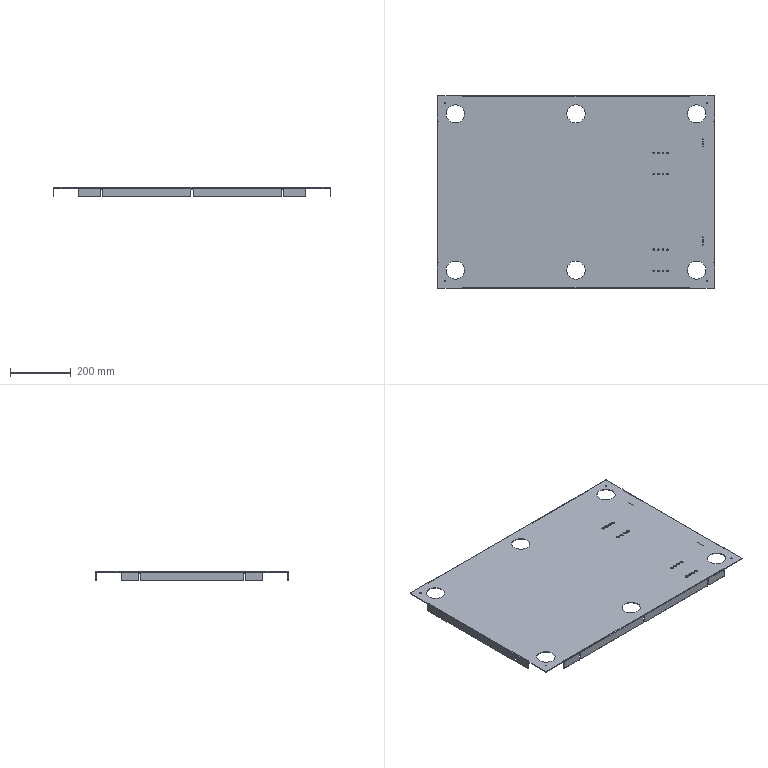Part | STEP file | 1 solid | 262 faces | box 918 x 636.5 x 30 mm | volume 1267450 mm3 | cylinder 154 | plane 108 | commonest cylinder face diameters 4 x32 5 x32 10.9 x32 2.5 x16 7 x14 60.5 x12